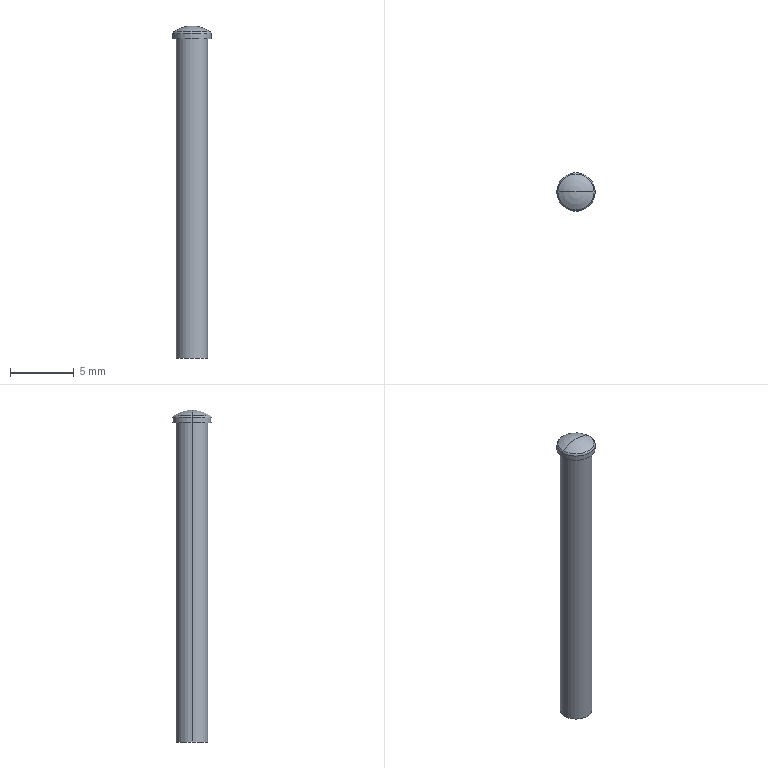Part | SolidWorks | features BaseBody 1 | 1 solid | 10 faces | box 3 x 3 x 26 mm | volume 128.07 mm3 | cylinder 4 | torus 2 | plane 2 | sphere 2 | commonest cylinder face diameters 2.5 x2 3 x2
STEP:
#1=CARTESIAN_POINT('',(-19.587,14.,0.5624));
#2=VERTEX_POINT('',#1);
#3=CARTESIAN_POINT('',(-19.5,14.,0.3974));
#4=VERTEX_POINT('',#3);
#5=CARTESIAN_POINT('',(-19.7,14.,0.3974));
#6=DIRECTION('',(0.,1.,0.));
#7=DIRECTION('',(-1.,0.,0.));
#8=AXIS2_PLACEMENT_3D('',#5,#6,#7);
#9=CIRCLE('',#8,0.2);
#10=EDGE_CURVE('',#2,#4,#9,.T.);
#11=ORIENTED_EDGE('',*,*,#10,.F.);
#12=CARTESIAN_POINT('',(-22.413,14.,0.5624));
#13=VERTEX_POINT('',#12);
#14=CARTESIAN_POINT('',(-21.,14.,0.5624));
#15=DIRECTION('',(0.,0.,1.));
#16=DIRECTION('',(-1.,0.,0.));
#17=AXIS2_PLACEMENT_3D('',#14,#15,#16);
#18=CIRCLE('',#17,1.413);
#19=EDGE_CURVE('',#13,#2,#18,.T.);
#20=ORIENTED_EDGE('',*,*,#19,.F.);
#21=CARTESIAN_POINT('',(-22.5,14.,0.3974));
#22=VERTEX_POINT('',#21);
#23=CARTESIAN_POINT('',(-22.3,14.,0.3974));
#24=DIRECTION('',(0.,-1.,0.));
#25=DIRECTION('',(0.,0.,-1.));
#26=AXIS2_PLACEMENT_3D('',#23,#24,#25);
#27=CIRCLE('',#26,0.2);
#28=EDGE_CURVE('',#13,#22,#27,.T.);
#29=ORIENTED_EDGE('',*,*,#28,.T.);
#30=CARTESIAN_POINT('',(-21.,14.,0.3974));
#31=DIRECTION('',(0.,0.,-1.));
#32=DIRECTION('',(-1.,0.,0.));
#33=AXIS2_PLACEMENT_3D('',#30,#31,#32);
#34=CIRCLE('',#33,1.5);
#35=EDGE_CURVE('',#4,#22,#34,.T.);
#36=ORIENTED_EDGE('',*,*,#35,.F.);
#37=EDGE_LOOP('',(#11,#20,#29,#36));
#38=FACE_OUTER_BOUND('',#37,.T.);
#39=CARTESIAN_POINT('',(-21.,14.,0.3974));
#40=DIRECTION('',(0.,0.,-1.));
#41=DIRECTION('',(-1.,0.,0.));
#42=AXIS2_PLACEMENT_3D('',#39,#40,#41);
#43=TOROIDAL_SURFACE('',#42,1.3,0.2);
#44=ADVANCED_FACE('',(#38),#43,.T.);
#45=CARTESIAN_POINT('',(-19.75,14.,0.));
#46=VERTEX_POINT('',#45);
#47=CARTESIAN_POINT('',(-22.25,14.,0.));
#48=VERTEX_POINT('',#47);
#49=CARTESIAN_POINT('',(-21.,14.,0.));
#50=DIRECTION('',(0.,0.,1.));
#51=DIRECTION('',(1.,0.,0.));
#52=AXIS2_PLACEMENT_3D('',#49,#50,#51);
#53=CIRCLE('',#52,1.25);
#54=EDGE_CURVE('',#46,#48,#53,.T.);
#55=ORIENTED_EDGE('',*,*,#54,.T.);
#56=CARTESIAN_POINT('',(-21.,14.,0.));
#57=DIRECTION('',(0.,0.,1.));
#58=DIRECTION('',(1.,0.,0.));
#59=AXIS2_PLACEMENT_3D('',#56,#57,#58);
#60=CIRCLE('',#59,1.25);
#61=EDGE_CURVE('',#48,#46,#60,.T.);
#62=ORIENTED_EDGE('',*,*,#61,.T.);
#63=EDGE_LOOP('',(#55,#62));
#64=FACE_BOUND('',#63,.T.);
#65=CARTESIAN_POINT('',(-22.5,14.,0.));
#66=VERTEX_POINT('',#65);
#67=CARTESIAN_POINT('',(-19.5,14.,0.));
#68=VERTEX_POINT('',#67);
#69=CARTESIAN_POINT('',(-21.,14.,0.));
#70=DIRECTION('',(0.,0.,1.));
#71=DIRECTION('',(1.,0.,0.));
#72=AXIS2_PLACEMENT_3D('',#69,#70,#71);
#73=CIRCLE('',#72,1.5);
#74=EDGE_CURVE('',#66,#68,#73,.T.);
#75=ORIENTED_EDGE('',*,*,#74,.F.);
#76=CARTESIAN_POINT('',(-21.,14.,0.));
#77=DIRECTION('',(0.,0.,1.));
#78=DIRECTION('',(1.,0.,0.));
#79=AXIS2_PLACEMENT_3D('',#76,#77,#78);
#80=CIRCLE('',#79,1.5);
#81=EDGE_CURVE('',#68,#66,#80,.T.);
#82=ORIENTED_EDGE('',*,*,#81,.F.);
#83=EDGE_LOOP('',(#75,#82));
#84=FACE_OUTER_BOUND('',#83,.T.);
#85=CARTESIAN_POINT('',(-21.,14.,0.));
#86=DIRECTION('',(0.,0.,1.));
#87=DIRECTION('',(1.,0.,0.));
#88=AXIS2_PLACEMENT_3D('',#85,#86,#87);
#89=PLANE('',#88);
#90=ADVANCED_FACE('',(#64,#84),#89,.F.);
#91=CARTESIAN_POINT('',(-21.,14.,-1.5));
#92=DIRECTION('',(0.,1.,0.));
#93=DIRECTION('',(-1.,0.,0.));
#94=AXIS2_PLACEMENT_3D('',#91,#92,#93);
#95=CIRCLE('',#94,2.5);
#96=EDGE_CURVE('',#13,#2,#95,.T.);
#97=ORIENTED_EDGE('',*,*,#96,.F.);
#98=ORIENTED_EDGE('',*,*,#19,.T.);
#99=EDGE_LOOP('',(#97,#98));
#100=FACE_OUTER_BOUND('',#99,.T.);
#101=CARTESIAN_POINT('',(-21.,14.,-1.5));
#102=DIRECTION('',(0.,0.,-1.));
#103=DIRECTION('',(1.,0.,0.));
#104=AXIS2_PLACEMENT_3D('',#101,#102,#103);
#105=SPHERICAL_SURFACE('',#104,2.5);
#106=ADVANCED_FACE('',(#100),#105,.T.);
#107=CARTESIAN_POINT('',(-19.5,14.,0.5));
#108=DIRECTION('',(0.,0.,-1.));
#109=VECTOR('',#108,1000.);
#110=LINE('',#107,#109);
#111=EDGE_CURVE('',#4,#68,#110,.T.);
#112=ORIENTED_EDGE('',*,*,#111,.F.);
#113=ORIENTED_EDGE('',*,*,#35,.T.);
#114=CARTESIAN_POINT('',(-22.5,14.,0.5));
#115=DIRECTION('',(0.,0.,-1.));
#116=VECTOR('',#115,1000.);
#117=LINE('',#114,#116);
#118=EDGE_CURVE('',#22,#66,#117,.T.);
#119=ORIENTED_EDGE('',*,*,#118,.T.);
#120=ORIENTED_EDGE('',*,*,#74,.T.);
#121=EDGE_LOOP('',(#112,#113,#119,#120));
#122=FACE_OUTER_BOUND('',#121,.T.);
#123=CARTESIAN_POINT('',(-21.,14.,0.5));
#124=DIRECTION('',(0.,0.,-1.));
#125=DIRECTION('',(-1.,0.,0.));
#126=AXIS2_PLACEMENT_3D('',#123,#124,#125);
#127=CYLINDRICAL_SURFACE('',#126,1.5);
#128=ADVANCED_FACE('',(#122),#127,.T.);
#129=CARTESIAN_POINT('',(-19.75,14.,-25.));
#130=VERTEX_POINT('',#129);
#131=CARTESIAN_POINT('',(-22.25,14.,-25.));
#132=VERTEX_POINT('',#131);
#133=CARTESIAN_POINT('',(-21.,14.,-25.));
#134=DIRECTION('',(0.,0.,1.));
#135=DIRECTION('',(1.,0.,0.));
#136=AXIS2_PLACEMENT_3D('',#133,#134,#135);
#137=CIRCLE('',#136,1.25);
#138=EDGE_CURVE('',#130,#132,#137,.T.);
#139=ORIENTED_EDGE('',*,*,#138,.F.);
#140=CARTESIAN_POINT('',(-21.,14.,-25.));
#141=DIRECTION('',(0.,0.,1.));
#142=DIRECTION('',(1.,0.,0.));
#143=AXIS2_PLACEMENT_3D('',#140,#141,#142);
#144=CIRCLE('',#143,1.25);
#145=EDGE_CURVE('',#132,#130,#144,.T.);
#146=ORIENTED_EDGE('',*,*,#145,.F.);
#147=EDGE_LOOP('',(#139,#146));
#148=FACE_OUTER_BOUND('',#147,.T.);
#149=CARTESIAN_POINT('',(-21.,14.,-25.));
#150=DIRECTION('',(0.,0.,1.));
#151=DIRECTION('',(1.,0.,0.));
#152=AXIS2_PLACEMENT_3D('',#149,#150,#151);
#153=PLANE('',#152);
#154=ADVANCED_FACE('',(#148),#153,.F.);
#155=CARTESIAN_POINT('',(-22.25,14.,-25.));
#156=DIRECTION('',(0.,0.,1.));
#157=VECTOR('',#156,1000.);
#158=LINE('',#155,#157);
#159=EDGE_CURVE('',#132,#48,#158,.T.);
#160=ORIENTED_EDGE('',*,*,#159,.F.);
#161=ORIENTED_EDGE('',*,*,#145,.T.);
#162=CARTESIAN_POINT('',(-19.75,14.,-25.));
#163=DIRECTION('',(0.,0.,1.));
#164=VECTOR('',#163,1000.);
#165=LINE('',#162,#164);
#166=EDGE_CURVE('',#130,#46,#165,.T.);
#167=ORIENTED_EDGE('',*,*,#166,.T.);
#168=ORIENTED_EDGE('',*,*,#61,.F.);
#169=EDGE_LOOP('',(#160,#161,#167,#168));
#170=FACE_OUTER_BOUND('',#169,.T.);
#171=CARTESIAN_POINT('',(-21.,14.,-25.));
#172=DIRECTION('',(0.,0.,1.));
#173=DIRECTION('',(1.,0.,0.));
#174=AXIS2_PLACEMENT_3D('',#171,#172,#173);
#175=CYLINDRICAL_SURFACE('',#174,1.25);
#176=ADVANCED_FACE('',(#170),#175,.T.);
#177=ORIENTED_EDGE('',*,*,#138,.T.);
#178=ORIENTED_EDGE('',*,*,#159,.T.);
#179=ORIENTED_EDGE('',*,*,#54,.F.);
#180=ORIENTED_EDGE('',*,*,#166,.F.);
#181=EDGE_LOOP('',(#177,#178,#179,#180));
#182=FACE_OUTER_BOUND('',#181,.T.);
#183=CARTESIAN_POINT('',(-21.,14.,-25.));
#184=DIRECTION('',(0.,0.,1.));
#185=DIRECTION('',(1.,0.,0.));
#186=AXIS2_PLACEMENT_3D('',#183,#184,#185);
#187=CYLINDRICAL_SURFACE('',#186,1.25);
#188=ADVANCED_FACE('',(#182),#187,.T.);
#189=CARTESIAN_POINT('',(-21.,14.,0.3974));
#190=DIRECTION('',(0.,0.,-1.));
#191=DIRECTION('',(-1.,0.,0.));
#192=AXIS2_PLACEMENT_3D('',#189,#190,#191);
#193=CIRCLE('',#192,1.5);
#194=EDGE_CURVE('',#22,#4,#193,.T.);
#195=ORIENTED_EDGE('',*,*,#194,.T.);
#196=ORIENTED_EDGE('',*,*,#111,.T.);
#197=ORIENTED_EDGE('',*,*,#81,.T.);
#198=ORIENTED_EDGE('',*,*,#118,.F.);
#199=EDGE_LOOP('',(#195,#196,#197,#198));
#200=FACE_OUTER_BOUND('',#199,.T.);
#201=CARTESIAN_POINT('',(-21.,14.,0.5));
#202=DIRECTION('',(0.,0.,-1.));
#203=DIRECTION('',(-1.,0.,0.));
#204=AXIS2_PLACEMENT_3D('',#201,#202,#203);
#205=CYLINDRICAL_SURFACE('',#204,1.5);
#206=ADVANCED_FACE('',(#200),#205,.T.);
#207=CARTESIAN_POINT('',(-21.,14.,0.5624));
#208=DIRECTION('',(0.,0.,1.));
#209=DIRECTION('',(-1.,0.,0.));
#210=AXIS2_PLACEMENT_3D('',#207,#208,#209);
#211=CIRCLE('',#210,1.413);
#212=EDGE_CURVE('',#2,#13,#211,.T.);
#213=ORIENTED_EDGE('',*,*,#212,.T.);
#214=ORIENTED_EDGE('',*,*,#96,.T.);
#215=EDGE_LOOP('',(#213,#214));
#216=FACE_OUTER_BOUND('',#215,.T.);
#217=CARTESIAN_POINT('',(-21.,14.,-1.5));
#218=DIRECTION('',(0.,0.,-1.));
#219=DIRECTION('',(1.,0.,0.));
#220=AXIS2_PLACEMENT_3D('',#217,#218,#219);
#221=SPHERICAL_SURFACE('',#220,2.5);
#222=ADVANCED_FACE('',(#216),#221,.T.);
#223=ORIENTED_EDGE('',*,*,#212,.F.);
#224=ORIENTED_EDGE('',*,*,#10,.T.);
#225=ORIENTED_EDGE('',*,*,#194,.F.);
#226=ORIENTED_EDGE('',*,*,#28,.F.);
#227=EDGE_LOOP('',(#223,#224,#225,#226));
#228=FACE_OUTER_BOUND('',#227,.T.);
#229=CARTESIAN_POINT('',(-21.,14.,0.3974));
#230=DIRECTION('',(0.,0.,-1.));
#231=DIRECTION('',(-1.,0.,0.));
#232=AXIS2_PLACEMENT_3D('',#229,#230,#231);
#233=TOROIDAL_SURFACE('',#232,1.3,0.2);
#234=ADVANCED_FACE('',(#228),#233,.T.);
#235=CLOSED_SHELL('',(#44,#90,#106,#128,#154,#176,#188,#206,#222,#234));
#236=MANIFOLD_SOLID_BREP('',#235);
#237=CARTESIAN_POINT('',(0.,0.,0.));
#238=DIRECTION('',(0.,0.,1.));
#239=DIRECTION('',(1.,0.,0.));
#240=AXIS2_PLACEMENT_3D('',#237,#238,#239);
#241=(LENGTH_UNIT()NAMED_UNIT(*)SI_UNIT(.MILLI.,.METRE.));
#242=UNCERTAINTY_MEASURE_WITH_UNIT(LENGTH_MEASURE(0.00001),#241,'','');
#243=(NAMED_UNIT(*)PLANE_ANGLE_UNIT()SI_UNIT($,.RADIAN.));
#244=(NAMED_UNIT(*)SI_UNIT($,.STERADIAN.)SOLID_ANGLE_UNIT());
#245=(GEOMETRIC_REPRESENTATION_CONTEXT(3)GLOBAL_UNCERTAINTY_ASSIGNED_CONTEXT((#242))GLOBAL_UNIT_ASSIGNED_CONTEXT((#241,#243,#244))REPRESENTATION_CONTEXT('',''));
#246=ADVANCED_BREP_SHAPE_REPRESENTATION('',(#236,#240),#245);